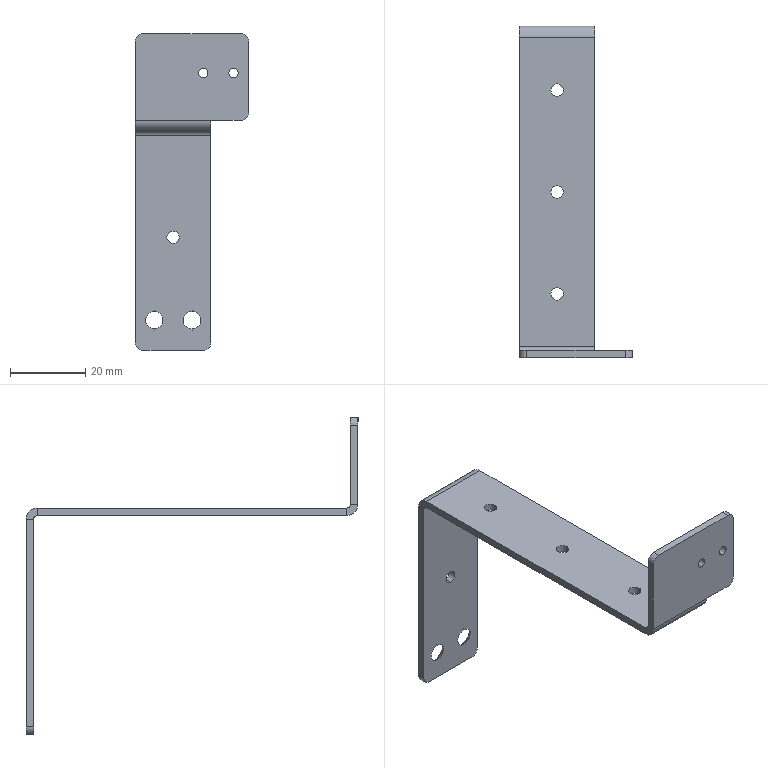Part | STEP file | FBDS-CS-014 | 1 solid | 44 faces | box 30 x 88 x 84 mm | volume 6954 mm3 | cylinder 21 | plane 19 | cone 4 | commonest cylinder face diameters 3.3 x8 4 x5 2.5 x4 2 x2 6 x2
STEP:
#1=CARTESIAN_POINT('',(0.,42.,-28.35));
#2=VERTEX_POINT('',#1);
#3=CARTESIAN_POINT('',(0.,42.,-31.65));
#4=VERTEX_POINT('',#3);
#5=CARTESIAN_POINT('',(0.,42.,-30.));
#6=DIRECTION('',(0.,-1.,0.));
#7=DIRECTION('',(0.,0.,-1.));
#8=AXIS2_PLACEMENT_3D('',#5,#6,#7);
#9=CIRCLE('',#8,1.65);
#10=EDGE_CURVE('',#2,#4,#9,.T.);
#11=ORIENTED_EDGE('',*,*,#10,.T.);
#12=CARTESIAN_POINT('',(0.,44.,-31.65));
#13=VERTEX_POINT('',#12);
#14=CARTESIAN_POINT('',(0.,44.,-31.65));
#15=DIRECTION('',(0.,1.,0.));
#16=VECTOR('',#15,1000.);
#17=LINE('',#14,#16);
#18=EDGE_CURVE('',#4,#13,#17,.T.);
#19=ORIENTED_EDGE('',*,*,#18,.T.);
#20=CARTESIAN_POINT('',(0.,44.,-28.35));
#21=VERTEX_POINT('',#20);
#22=CARTESIAN_POINT('',(0.,44.,-30.));
#23=DIRECTION('',(0.,1.,0.));
#24=DIRECTION('',(0.,0.,1.));
#25=AXIS2_PLACEMENT_3D('',#22,#23,#24);
#26=CIRCLE('',#25,1.65);
#27=EDGE_CURVE('',#13,#21,#26,.T.);
#28=ORIENTED_EDGE('',*,*,#27,.T.);
#29=CARTESIAN_POINT('',(0.,44.,-28.35));
#30=DIRECTION('',(0.,1.,0.));
#31=VECTOR('',#30,1000.);
#32=LINE('',#29,#31);
#33=EDGE_CURVE('',#2,#21,#32,.T.);
#34=ORIENTED_EDGE('',*,*,#33,.F.);
#35=EDGE_LOOP('',(#11,#19,#28,#34));
#36=FACE_OUTER_BOUND('',#35,.T.);
#37=CARTESIAN_POINT('',(0.,44.,-30.));
#38=DIRECTION('',(0.,1.,0.));
#39=DIRECTION('',(0.,0.,1.));
#40=AXIS2_PLACEMENT_3D('',#37,#38,#39);
#41=CYLINDRICAL_SURFACE('',#40,1.65);
#42=ADVANCED_FACE('',(#36),#41,.F.);
#43=CARTESIAN_POINT('',(1.65,27.,-2.));
#44=VERTEX_POINT('',#43);
#45=CARTESIAN_POINT('',(-1.65,27.,-2.));
#46=VERTEX_POINT('',#45);
#47=CARTESIAN_POINT('',(0.,27.,-2.));
#48=DIRECTION('',(0.,0.,-1.));
#49=DIRECTION('',(-1.,0.,0.));
#50=AXIS2_PLACEMENT_3D('',#47,#48,#49);
#51=CIRCLE('',#50,1.65);
#52=EDGE_CURVE('',#44,#46,#51,.T.);
#53=ORIENTED_EDGE('',*,*,#52,.T.);
#54=CARTESIAN_POINT('',(-1.65,27.,0.));
#55=VERTEX_POINT('',#54);
#56=CARTESIAN_POINT('',(-1.65,27.,0.));
#57=DIRECTION('',(0.,0.,1.));
#58=VECTOR('',#57,1000.);
#59=LINE('',#56,#58);
#60=EDGE_CURVE('',#46,#55,#59,.T.);
#61=ORIENTED_EDGE('',*,*,#60,.T.);
#62=CARTESIAN_POINT('',(1.65,27.,0.));
#63=VERTEX_POINT('',#62);
#64=CARTESIAN_POINT('',(0.,27.,0.));
#65=DIRECTION('',(0.,0.,1.));
#66=DIRECTION('',(1.,0.,0.));
#67=AXIS2_PLACEMENT_3D('',#64,#65,#66);
#68=CIRCLE('',#67,1.65);
#69=EDGE_CURVE('',#55,#63,#68,.T.);
#70=ORIENTED_EDGE('',*,*,#69,.T.);
#71=CARTESIAN_POINT('',(1.65,27.,0.));
#72=DIRECTION('',(0.,0.,1.));
#73=VECTOR('',#72,1000.);
#74=LINE('',#71,#73);
#75=EDGE_CURVE('',#44,#63,#74,.T.);
#76=ORIENTED_EDGE('',*,*,#75,.F.);
#77=EDGE_LOOP('',(#53,#61,#70,#76));
#78=FACE_OUTER_BOUND('',#77,.T.);
#79=CARTESIAN_POINT('',(0.,27.,0.));
#80=DIRECTION('',(0.,0.,1.));
#81=DIRECTION('',(1.,0.,0.));
#82=AXIS2_PLACEMENT_3D('',#79,#80,#81);
#83=CYLINDRICAL_SURFACE('',#82,1.65);
#84=ADVANCED_FACE('',(#78),#83,.F.);
#85=CARTESIAN_POINT('',(1.65,0.,-2.));
#86=VERTEX_POINT('',#85);
#87=CARTESIAN_POINT('',(-1.65,0.,-2.));
#88=VERTEX_POINT('',#87);
#89=CARTESIAN_POINT('',(0.,0.,-2.));
#90=DIRECTION('',(0.,0.,-1.));
#91=DIRECTION('',(-1.,0.,0.));
#92=AXIS2_PLACEMENT_3D('',#89,#90,#91);
#93=CIRCLE('',#92,1.65);
#94=EDGE_CURVE('',#86,#88,#93,.T.);
#95=ORIENTED_EDGE('',*,*,#94,.T.);
#96=CARTESIAN_POINT('',(-1.65,0.,0.));
#97=VERTEX_POINT('',#96);
#98=CARTESIAN_POINT('',(-1.65,0.,0.));
#99=DIRECTION('',(0.,0.,1.));
#100=VECTOR('',#99,1000.);
#101=LINE('',#98,#100);
#102=EDGE_CURVE('',#88,#97,#101,.T.);
#103=ORIENTED_EDGE('',*,*,#102,.T.);
#104=CARTESIAN_POINT('',(1.65,0.,0.));
#105=VERTEX_POINT('',#104);
#106=CARTESIAN_POINT('',(0.,0.,0.));
#107=DIRECTION('',(0.,0.,1.));
#108=DIRECTION('',(1.,0.,0.));
#109=AXIS2_PLACEMENT_3D('',#106,#107,#108);
#110=CIRCLE('',#109,1.65);
#111=EDGE_CURVE('',#97,#105,#110,.T.);
#112=ORIENTED_EDGE('',*,*,#111,.T.);
#113=CARTESIAN_POINT('',(1.65,0.,0.));
#114=DIRECTION('',(0.,0.,1.));
#115=VECTOR('',#114,1000.);
#116=LINE('',#113,#115);
#117=EDGE_CURVE('',#86,#105,#116,.T.);
#118=ORIENTED_EDGE('',*,*,#117,.F.);
#119=EDGE_LOOP('',(#95,#103,#112,#118));
#120=FACE_OUTER_BOUND('',#119,.T.);
#121=CARTESIAN_POINT('',(0.,0.,0.));
#122=DIRECTION('',(0.,0.,1.));
#123=DIRECTION('',(1.,0.,0.));
#124=AXIS2_PLACEMENT_3D('',#121,#122,#123);
#125=CYLINDRICAL_SURFACE('',#124,1.65);
#126=ADVANCED_FACE('',(#120),#125,.F.);
#127=CARTESIAN_POINT('',(1.65,-27.,-2.));
#128=VERTEX_POINT('',#127);
#129=CARTESIAN_POINT('',(-1.65,-27.,-2.));
#130=VERTEX_POINT('',#129);
#131=CARTESIAN_POINT('',(0.,-27.,-2.));
#132=DIRECTION('',(0.,0.,-1.));
#133=DIRECTION('',(-1.,0.,0.));
#134=AXIS2_PLACEMENT_3D('',#131,#132,#133);
#135=CIRCLE('',#134,1.65);
#136=EDGE_CURVE('',#128,#130,#135,.T.);
#137=ORIENTED_EDGE('',*,*,#136,.T.);
#138=CARTESIAN_POINT('',(-1.65,-27.,0.));
#139=VERTEX_POINT('',#138);
#140=CARTESIAN_POINT('',(-1.65,-27.,0.));
#141=DIRECTION('',(0.,0.,1.));
#142=VECTOR('',#141,1000.);
#143=LINE('',#140,#142);
#144=EDGE_CURVE('',#130,#139,#143,.T.);
#145=ORIENTED_EDGE('',*,*,#144,.T.);
#146=CARTESIAN_POINT('',(1.65,-27.,0.));
#147=VERTEX_POINT('',#146);
#148=CARTESIAN_POINT('',(0.,-27.,0.));
#149=DIRECTION('',(0.,0.,1.));
#150=DIRECTION('',(1.,0.,0.));
#151=AXIS2_PLACEMENT_3D('',#148,#149,#150);
#152=CIRCLE('',#151,1.65);
#153=EDGE_CURVE('',#139,#147,#152,.T.);
#154=ORIENTED_EDGE('',*,*,#153,.T.);
#155=CARTESIAN_POINT('',(1.65,-27.,0.));
#156=DIRECTION('',(0.,0.,1.));
#157=VECTOR('',#156,1000.);
#158=LINE('',#155,#157);
#159=EDGE_CURVE('',#128,#147,#158,.T.);
#160=ORIENTED_EDGE('',*,*,#159,.F.);
#161=EDGE_LOOP('',(#137,#145,#154,#160));
#162=FACE_OUTER_BOUND('',#161,.T.);
#163=CARTESIAN_POINT('',(0.,-27.,0.));
#164=DIRECTION('',(0.,0.,1.));
#165=DIRECTION('',(1.,0.,0.));
#166=AXIS2_PLACEMENT_3D('',#163,#164,#165);
#167=CYLINDRICAL_SURFACE('',#166,1.65);
#168=ADVANCED_FACE('',(#162),#167,.F.);
#169=CARTESIAN_POINT('',(16.,-44.,12.25));
#170=VERTEX_POINT('',#169);
#171=CARTESIAN_POINT('',(16.,-44.,14.75));
#172=VERTEX_POINT('',#171);
#173=CARTESIAN_POINT('',(16.,-44.,13.5));
#174=DIRECTION('',(0.,1.,0.));
#175=DIRECTION('',(0.,0.,1.));
#176=AXIS2_PLACEMENT_3D('',#173,#174,#175);
#177=CIRCLE('',#176,1.25);
#178=EDGE_CURVE('',#170,#172,#177,.T.);
#179=ORIENTED_EDGE('',*,*,#178,.F.);
#180=CARTESIAN_POINT('',(16.,-42.,12.25));
#181=VERTEX_POINT('',#180);
#182=CARTESIAN_POINT('',(16.,-42.,12.25));
#183=DIRECTION('',(0.,1.,0.));
#184=VECTOR('',#183,1000.);
#185=LINE('',#182,#184);
#186=EDGE_CURVE('',#170,#181,#185,.T.);
#187=ORIENTED_EDGE('',*,*,#186,.T.);
#188=CARTESIAN_POINT('',(16.,-42.,14.75));
#189=VERTEX_POINT('',#188);
#190=CARTESIAN_POINT('',(16.,-42.,13.5));
#191=DIRECTION('',(0.,1.,0.));
#192=DIRECTION('',(0.,0.,1.));
#193=AXIS2_PLACEMENT_3D('',#190,#191,#192);
#194=CIRCLE('',#193,1.25);
#195=EDGE_CURVE('',#181,#189,#194,.T.);
#196=ORIENTED_EDGE('',*,*,#195,.T.);
#197=CARTESIAN_POINT('',(16.,-42.,14.75));
#198=DIRECTION('',(0.,1.,0.));
#199=VECTOR('',#198,1000.);
#200=LINE('',#197,#199);
#201=EDGE_CURVE('',#172,#189,#200,.T.);
#202=ORIENTED_EDGE('',*,*,#201,.F.);
#203=EDGE_LOOP('',(#179,#187,#196,#202));
#204=FACE_OUTER_BOUND('',#203,.T.);
#205=CARTESIAN_POINT('',(16.,-42.,13.5));
#206=DIRECTION('',(0.,1.,0.));
#207=DIRECTION('',(0.,0.,1.));
#208=AXIS2_PLACEMENT_3D('',#205,#206,#207);
#209=CYLINDRICAL_SURFACE('',#208,1.25);
#210=ADVANCED_FACE('',(#204),#209,.F.);
#211=CARTESIAN_POINT('',(8.,-44.,12.25));
#212=VERTEX_POINT('',#211);
#213=CARTESIAN_POINT('',(8.,-44.,14.75));
#214=VERTEX_POINT('',#213);
#215=CARTESIAN_POINT('',(8.,-44.,13.5));
#216=DIRECTION('',(0.,1.,0.));
#217=DIRECTION('',(0.,0.,1.));
#218=AXIS2_PLACEMENT_3D('',#215,#216,#217);
#219=CIRCLE('',#218,1.25);
#220=EDGE_CURVE('',#212,#214,#219,.T.);
#221=ORIENTED_EDGE('',*,*,#220,.F.);
#222=CARTESIAN_POINT('',(8.,-42.,12.25));
#223=VERTEX_POINT('',#222);
#224=CARTESIAN_POINT('',(8.,-42.,12.25));
#225=DIRECTION('',(0.,1.,0.));
#226=VECTOR('',#225,1000.);
#227=LINE('',#224,#226);
#228=EDGE_CURVE('',#212,#223,#227,.T.);
#229=ORIENTED_EDGE('',*,*,#228,.T.);
#230=CARTESIAN_POINT('',(8.,-42.,14.75));
#231=VERTEX_POINT('',#230);
#232=CARTESIAN_POINT('',(8.,-42.,13.5));
#233=DIRECTION('',(0.,1.,0.));
#234=DIRECTION('',(0.,0.,1.));
#235=AXIS2_PLACEMENT_3D('',#232,#233,#234);
#236=CIRCLE('',#235,1.25);
#237=EDGE_CURVE('',#223,#231,#236,.T.);
#238=ORIENTED_EDGE('',*,*,#237,.T.);
#239=CARTESIAN_POINT('',(8.,-42.,14.75));
#240=DIRECTION('',(0.,1.,0.));
#241=VECTOR('',#240,1000.);
#242=LINE('',#239,#241);
#243=EDGE_CURVE('',#214,#231,#242,.T.);
#244=ORIENTED_EDGE('',*,*,#243,.F.);
#245=EDGE_LOOP('',(#221,#229,#238,#244));
#246=FACE_OUTER_BOUND('',#245,.T.);
#247=CARTESIAN_POINT('',(8.,-42.,13.5));
#248=DIRECTION('',(0.,1.,0.));
#249=DIRECTION('',(0.,0.,1.));
#250=AXIS2_PLACEMENT_3D('',#247,#248,#249);
#251=CYLINDRICAL_SURFACE('',#250,1.25);
#252=ADVANCED_FACE('',(#246),#251,.F.);
#253=CARTESIAN_POINT('',(-5.,42.,-49.7));
#254=VERTEX_POINT('',#253);
#255=CARTESIAN_POINT('',(-5.,42.,-54.3));
#256=VERTEX_POINT('',#255);
#257=CARTESIAN_POINT('',(-5.,42.,-52.));
#258=DIRECTION('',(0.,-1.,0.));
#259=DIRECTION('',(0.,0.,-1.));
#260=AXIS2_PLACEMENT_3D('',#257,#258,#259);
#261=CIRCLE('',#260,2.3);
#262=EDGE_CURVE('',#254,#256,#261,.T.);
#263=ORIENTED_EDGE('',*,*,#262,.T.);
#264=CARTESIAN_POINT('',(-5.,44.,-56.3));
#265=VERTEX_POINT('',#264);
#266=CARTESIAN_POINT('',(-5.,44.,-56.3));
#267=DIRECTION('',(0.,0.7071,-0.7071));
#268=VECTOR('',#267,1000.);
#269=LINE('',#266,#268);
#270=EDGE_CURVE('',#256,#265,#269,.T.);
#271=ORIENTED_EDGE('',*,*,#270,.T.);
#272=CARTESIAN_POINT('',(-5.,44.,-47.7));
#273=VERTEX_POINT('',#272);
#274=CARTESIAN_POINT('',(-5.,44.,-52.));
#275=DIRECTION('',(0.,1.,0.));
#276=DIRECTION('',(0.,0.,1.));
#277=AXIS2_PLACEMENT_3D('',#274,#275,#276);
#278=CIRCLE('',#277,4.3);
#279=EDGE_CURVE('',#265,#273,#278,.T.);
#280=ORIENTED_EDGE('',*,*,#279,.T.);
#281=CARTESIAN_POINT('',(-5.,44.,-47.7));
#282=DIRECTION('',(0.,0.7071,0.7071));
#283=VECTOR('',#282,1000.);
#284=LINE('',#281,#283);
#285=EDGE_CURVE('',#254,#273,#284,.T.);
#286=ORIENTED_EDGE('',*,*,#285,.F.);
#287=EDGE_LOOP('',(#263,#271,#280,#286));
#288=FACE_OUTER_BOUND('',#287,.T.);
#289=CARTESIAN_POINT('',(-5.,44.,-52.));
#290=DIRECTION('',(0.,1.,0.));
#291=DIRECTION('',(0.,0.,1.));
#292=AXIS2_PLACEMENT_3D('',#289,#290,#291);
#293=CONICAL_SURFACE('',#292,4.3,0.7854);
#294=ADVANCED_FACE('',(#288),#293,.F.);
#295=CARTESIAN_POINT('',(5.,42.,-49.7));
#296=VERTEX_POINT('',#295);
#297=CARTESIAN_POINT('',(5.,42.,-54.3));
#298=VERTEX_POINT('',#297);
#299=CARTESIAN_POINT('',(5.,42.,-52.));
#300=DIRECTION('',(0.,-1.,0.));
#301=DIRECTION('',(0.,0.,-1.));
#302=AXIS2_PLACEMENT_3D('',#299,#300,#301);
#303=CIRCLE('',#302,2.3);
#304=EDGE_CURVE('',#296,#298,#303,.T.);
#305=ORIENTED_EDGE('',*,*,#304,.T.);
#306=CARTESIAN_POINT('',(5.,44.,-56.3));
#307=VERTEX_POINT('',#306);
#308=CARTESIAN_POINT('',(5.,44.,-56.3));
#309=DIRECTION('',(0.,0.7071,-0.7071));
#310=VECTOR('',#309,1000.);
#311=LINE('',#308,#310);
#312=EDGE_CURVE('',#298,#307,#311,.T.);
#313=ORIENTED_EDGE('',*,*,#312,.T.);
#314=CARTESIAN_POINT('',(5.,44.,-47.7));
#315=VERTEX_POINT('',#314);
#316=CARTESIAN_POINT('',(5.,44.,-52.));
#317=DIRECTION('',(0.,1.,0.));
#318=DIRECTION('',(0.,0.,1.));
#319=AXIS2_PLACEMENT_3D('',#316,#317,#318);
#320=CIRCLE('',#319,4.3);
#321=EDGE_CURVE('',#307,#315,#320,.T.);
#322=ORIENTED_EDGE('',*,*,#321,.T.);
#323=CARTESIAN_POINT('',(5.,44.,-47.7));
#324=DIRECTION('',(0.,0.7071,0.7071));
#325=VECTOR('',#324,1000.);
#326=LINE('',#323,#325);
#327=EDGE_CURVE('',#296,#315,#326,.T.);
#328=ORIENTED_EDGE('',*,*,#327,.F.);
#329=EDGE_LOOP('',(#305,#313,#322,#328));
#330=FACE_OUTER_BOUND('',#329,.T.);
#331=CARTESIAN_POINT('',(5.,44.,-52.));
#332=DIRECTION('',(0.,1.,0.));
#333=DIRECTION('',(0.,0.,1.));
#334=AXIS2_PLACEMENT_3D('',#331,#332,#333);
#335=CONICAL_SURFACE('',#334,4.3,0.7854);
#336=ADVANCED_FACE('',(#330),#335,.F.);
#337=CARTESIAN_POINT('',(10.,-41.,0.));
#338=VERTEX_POINT('',#337);
#339=CARTESIAN_POINT('',(10.,41.,0.));
#340=VERTEX_POINT('',#339);
#341=CARTESIAN_POINT('',(10.,-42.,0.));
#342=DIRECTION('',(0.,1.,0.));
#343=VECTOR('',#342,1000.);
#344=LINE('',#341,#343);
#345=EDGE_CURVE('',#338,#340,#344,.T.);
#346=ORIENTED_EDGE('',*,*,#345,.F.);
#347=CARTESIAN_POINT('',(10.,-41.,-2.));
#348=VERTEX_POINT('',#347);
#349=CARTESIAN_POINT('',(10.,-41.,0.));
#350=DIRECTION('',(0.,0.,-1.));
#351=VECTOR('',#350,1000.);
#352=LINE('',#349,#351);
#353=EDGE_CURVE('',#338,#348,#352,.T.);
#354=ORIENTED_EDGE('',*,*,#353,.T.);
#355=CARTESIAN_POINT('',(10.,41.,-2.));
#356=VERTEX_POINT('',#355);
#357=CARTESIAN_POINT('',(10.,-42.,-2.));
#358=DIRECTION('',(0.,1.,0.));
#359=VECTOR('',#358,1000.);
#360=LINE('',#357,#359);
#361=EDGE_CURVE('',#348,#356,#360,.T.);
#362=ORIENTED_EDGE('',*,*,#361,.T.);
#363=CARTESIAN_POINT('',(10.,41.,-2.));
#364=DIRECTION('',(0.,0.,1.));
#365=VECTOR('',#364,1000.);
#366=LINE('',#363,#365);
#367=EDGE_CURVE('',#356,#340,#366,.T.);
#368=ORIENTED_EDGE('',*,*,#367,.T.);
#369=EDGE_LOOP('',(#346,#354,#362,#368));
#370=FACE_OUTER_BOUND('',#369,.T.);
#371=CARTESIAN_POINT('',(10.,-42.,-2.));
#372=DIRECTION('',(1.,0.,0.));
#373=DIRECTION('',(0.,0.,-1.));
#374=AXIS2_PLACEMENT_3D('',#371,#372,#373);
#375=PLANE('',#374);
#376=ADVANCED_FACE('',(#370),#375,.T.);
#377=ORIENTED_EDGE('',*,*,#52,.F.);
#378=CARTESIAN_POINT('',(0.,27.,-2.));
#379=DIRECTION('',(0.,0.,-1.));
#380=DIRECTION('',(-1.,0.,0.));
#381=AXIS2_PLACEMENT_3D('',#378,#379,#380);
#382=CIRCLE('',#381,1.65);
#383=EDGE_CURVE('',#46,#44,#382,.T.);
#384=ORIENTED_EDGE('',*,*,#383,.F.);
#385=EDGE_LOOP('',(#377,#384));
#386=FACE_BOUND('',#385,.T.);
#387=ORIENTED_EDGE('',*,*,#94,.F.);
#388=CARTESIAN_POINT('',(0.,0.,-2.));
#389=DIRECTION('',(0.,0.,-1.));
#390=DIRECTION('',(-1.,0.,0.));
#391=AXIS2_PLACEMENT_3D('',#388,#389,#390);
#392=CIRCLE('',#391,1.65);
#393=EDGE_CURVE('',#88,#86,#392,.T.);
#394=ORIENTED_EDGE('',*,*,#393,.F.);
#395=EDGE_LOOP('',(#387,#394));
#396=FACE_BOUND('',#395,.T.);
#397=ORIENTED_EDGE('',*,*,#136,.F.);
#398=CARTESIAN_POINT('',(0.,-27.,-2.));
#399=DIRECTION('',(0.,0.,-1.));
#400=DIRECTION('',(-1.,0.,0.));
#401=AXIS2_PLACEMENT_3D('',#398,#399,#400);
#402=CIRCLE('',#401,1.65);
#403=EDGE_CURVE('',#130,#128,#402,.T.);
#404=ORIENTED_EDGE('',*,*,#403,.F.);
#405=EDGE_LOOP('',(#397,#404));
#406=FACE_BOUND('',#405,.T.);
#407=ORIENTED_EDGE('',*,*,#361,.F.);
#408=CARTESIAN_POINT('',(-10.,-41.,-2.));
#409=VERTEX_POINT('',#408);
#410=CARTESIAN_POINT('',(10.,-41.,-2.));
#411=DIRECTION('',(-1.,0.,0.));
#412=VECTOR('',#411,1000.);
#413=LINE('',#410,#412);
#414=EDGE_CURVE('',#348,#409,#413,.T.);
#415=ORIENTED_EDGE('',*,*,#414,.T.);
#416=CARTESIAN_POINT('',(-10.,41.,-2.));
#417=VERTEX_POINT('',#416);
#418=CARTESIAN_POINT('',(-10.,-42.,-2.));
#419=DIRECTION('',(0.,-1.,0.));
#420=VECTOR('',#419,1000.);
#421=LINE('',#418,#420);
#422=EDGE_CURVE('',#417,#409,#421,.T.);
#423=ORIENTED_EDGE('',*,*,#422,.F.);
#424=CARTESIAN_POINT('',(10.,41.,-2.));
#425=DIRECTION('',(-1.,0.,0.));
#426=VECTOR('',#425,1000.);
#427=LINE('',#424,#426);
#428=EDGE_CURVE('',#356,#417,#427,.T.);
#429=ORIENTED_EDGE('',*,*,#428,.F.);
#430=EDGE_LOOP('',(#407,#415,#423,#429));
#431=FACE_OUTER_BOUND('',#430,.T.);
#432=CARTESIAN_POINT('',(0.,0.,-2.));
#433=DIRECTION('',(0.,0.,-1.));
#434=DIRECTION('',(-1.,0.,0.));
#435=AXIS2_PLACEMENT_3D('',#432,#433,#434);
#436=PLANE('',#435);
#437=ADVANCED_FACE('',(#386,#396,#406,#431),#436,.T.);
#438=CARTESIAN_POINT('',(0.,27.,0.));
#439=DIRECTION('',(0.,0.,1.));
#440=DIRECTION('',(1.,0.,0.));
#441=AXIS2_PLACEMENT_3D('',#438,#439,#440);
#442=CIRCLE('',#441,1.65);
#443=EDGE_CURVE('',#63,#55,#442,.T.);
#444=ORIENTED_EDGE('',*,*,#443,.F.);
#445=ORIENTED_EDGE('',*,*,#69,.F.);
#446=EDGE_LOOP('',(#444,#445));
#447=FACE_BOUND('',#446,.T.);
#448=CARTESIAN_POINT('',(0.,0.,0.));
#449=DIRECTION('',(0.,0.,1.));
#450=DIRECTION('',(1.,0.,0.));
#451=AXIS2_PLACEMENT_3D('',#448,#449,#450);
#452=CIRCLE('',#451,1.65);
#453=EDGE_CURVE('',#105,#97,#452,.T.);
#454=ORIENTED_EDGE('',*,*,#453,.F.);
#455=ORIENTED_EDGE('',*,*,#111,.F.);
#456=EDGE_LOOP('',(#454,#455));
#457=FACE_BOUND('',#456,.T.);
#458=CARTESIAN_POINT('',(0.,-27.,0.));
#459=DIRECTION('',(0.,0.,1.));
#460=DIRECTION('',(1.,0.,0.));
#461=AXIS2_PLACEMENT_3D('',#458,#459,#460);
#462=CIRCLE('',#461,1.65);
#463=EDGE_CURVE('',#147,#139,#462,.T.);
#464=ORIENTED_EDGE('',*,*,#463,.F.);
#465=ORIENTED_EDGE('',*,*,#153,.F.);
#466=EDGE_LOOP('',(#464,#465));
#467=FACE_BOUND('',#466,.T.);
#468=CARTESIAN_POINT('',(-10.,-41.,0.));
#469=VERTEX_POINT('',#468);
#470=CARTESIAN_POINT('',(10.,-41.,0.));
#471=DIRECTION('',(-1.,0.,0.));
#472=VECTOR('',#471,1000.);
#473=LINE('',#470,#472);
#474=EDGE_CURVE('',#338,#469,#473,.T.);
#475=ORIENTED_EDGE('',*,*,#474,.F.);
#476=ORIENTED_EDGE('',*,*,#345,.T.);
#477=CARTESIAN_POINT('',(-10.,41.,0.));
#478=VERTEX_POINT('',#477);
#479=CARTESIAN_POINT('',(10.,41.,0.));
#480=DIRECTION('',(-1.,0.,0.));
#481=VECTOR('',#480,1000.);
#482=LINE('',#479,#481);
#483=EDGE_CURVE('',#340,#478,#482,.T.);
#484=ORIENTED_EDGE('',*,*,#483,.T.);
#485=CARTESIAN_POINT('',(-10.,-42.,0.));
#486=DIRECTION('',(0.,-1.,0.));
#487=VECTOR('',#486,1000.);
#488=LINE('',#485,#487);
#489=EDGE_CURVE('',#478,#469,#488,.T.);
#490=ORIENTED_EDGE('',*,*,#489,.T.);
#491=EDGE_LOOP('',(#475,#476,#484,#490));
#492=FACE_OUTER_BOUND('',#491,.T.);
#493=CARTESIAN_POINT('',(0.,0.,0.));
#494=DIRECTION('',(0.,0.,-1.));
#495=DIRECTION('',(-1.,0.,0.));
#496=AXIS2_PLACEMENT_3D('',#493,#494,#495);
#497=PLANE('',#496);
#498=ADVANCED_FACE('',(#447,#457,#467,#492),#497,.F.);
#499=CARTESIAN_POINT('',(-10.,-41.,0.));
#500=DIRECTION('',(0.,0.,-1.));
#501=VECTOR('',#500,1000.);
#502=LINE('',#499,#501);
#503=EDGE_CURVE('',#469,#409,#502,.T.);
#504=ORIENTED_EDGE('',*,*,#503,.F.);
#505=ORIENTED_EDGE('',*,*,#489,.F.);
#506=CARTESIAN_POINT('',(-10.,41.,-2.));
#507=DIRECTION('',(0.,0.,1.));
#508=VECTOR('',#507,1000.);
#509=LINE('',#506,#508);
#510=EDGE_CURVE('',#417,#478,#509,.T.);
#511=ORIENTED_EDGE('',*,*,#510,.F.);
#512=ORIENTED_EDGE('',*,*,#422,.T.);
#513=EDGE_LOOP('',(#504,#505,#511,#512));
#514=FACE_OUTER_BOUND('',#513,.T.);
#515=CARTESIAN_POINT('',(-10.,-42.,-2.));
#516=DIRECTION('',(-1.,0.,0.));
#517=DIRECTION('',(0.,0.,1.));
#518=AXIS2_PLACEMENT_3D('',#515,#516,#517);
#519=PLANE('',#518);
#520=ADVANCED_FACE('',(#514),#519,.T.);
#521=CARTESIAN_POINT('',(-10.,42.,-3.));
#522=VERTEX_POINT('',#521);
#523=CARTESIAN_POINT('',(-10.,44.,-3.));
#524=VERTEX_POINT('',#523);
#525=CARTESIAN_POINT('',(-10.,42.,-3.));
#526=DIRECTION('',(0.,1.,0.));
#527=VECTOR('',#526,1000.);
#528=LINE('',#525,#527);
#529=EDGE_CURVE('',#522,#524,#528,.T.);
#530=ORIENTED_EDGE('',*,*,#529,.F.);
#531=CARTESIAN_POINT('',(-10.,41.,-3.));
#532=DIRECTION('',(-1.,0.,0.));
#533=DIRECTION('',(0.,0.,-1.));
#534=AXIS2_PLACEMENT_3D('',#531,#532,#533);
#535=CIRCLE('',#534,1.);
#536=EDGE_CURVE('',#417,#522,#535,.T.);
#537=ORIENTED_EDGE('',*,*,#536,.F.);
#538=ORIENTED_EDGE('',*,*,#510,.T.);
#539=CARTESIAN_POINT('',(-10.,41.,-3.));
#540=DIRECTION('',(-1.,0.,0.));
#541=DIRECTION('',(0.,0.,-1.));
#542=AXIS2_PLACEMENT_3D('',#539,#540,#541);
#543=CIRCLE('',#542,3.);
#544=EDGE_CURVE('',#478,#524,#543,.T.);
#545=ORIENTED_EDGE('',*,*,#544,.T.);
#546=EDGE_LOOP('',(#530,#537,#538,#545));
#547=FACE_OUTER_BOUND('',#546,.T.);
#548=CARTESIAN_POINT('',(-10.,41.,-3.));
#549=DIRECTION('',(-1.,0.,0.));
#550=DIRECTION('',(0.,0.,1.));
#551=AXIS2_PLACEMENT_3D('',#548,#549,#550);
#552=PLANE('',#551);
#553=ADVANCED_FACE('',(#547),#552,.T.);
#554=CARTESIAN_POINT('',(10.,42.,-3.));
#555=VERTEX_POINT('',#554);
#556=CARTESIAN_POINT('',(10.,41.,-3.));
#557=DIRECTION('',(1.,0.,0.));
#558=DIRECTION('',(0.,0.,-1.));
#559=AXIS2_PLACEMENT_3D('',#556,#557,#558);
#560=CIRCLE('',#559,1.);
#561=EDGE_CURVE('',#555,#356,#560,.T.);
#562=ORIENTED_EDGE('',*,*,#561,.F.);
#563=CARTESIAN_POINT('',(10.,44.,-3.));
#564=VERTEX_POINT('',#563);
#565=CARTESIAN_POINT('',(10.,42.,-3.));
#566=DIRECTION('',(0.,1.,0.));
#567=VECTOR('',#566,1000.);
#568=LINE('',#565,#567);
#569=EDGE_CURVE('',#555,#564,#568,.T.);
#570=ORIENTED_EDGE('',*,*,#569,.T.);
#571=CARTESIAN_POINT('',(10.,41.,-3.));
#572=DIRECTION('',(1.,0.,0.));
#573=DIRECTION('',(0.,0.,-1.));
#574=AXIS2_PLACEMENT_3D('',#571,#572,#573);
#575=CIRCLE('',#574,3.);
#576=EDGE_CURVE('',#564,#340,#575,.T.);
#577=ORIENTED_EDGE('',*,*,#576,.T.);
#578=ORIENTED_EDGE('',*,*,#367,.F.);
#579=EDGE_LOOP('',(#562,#570,#577,#578));
#580=FACE_OUTER_BOUND('',#579,.T.);
#581=CARTESIAN_POINT('',(10.,41.,-3.));
#582=DIRECTION('',(-1.,0.,0.));
#583=DIRECTION('',(0.,0.,1.));
#584=AXIS2_PLACEMENT_3D('',#581,#582,#583);
#585=PLANE('',#584);
#586=ADVANCED_FACE('',(#580),#585,.F.);
#587=ORIENTED_EDGE('',*,*,#483,.F.);
#588=ORIENTED_EDGE('',*,*,#576,.F.);
#589=CARTESIAN_POINT('',(0.,44.,-3.));
#590=DIRECTION('',(-1.,0.,0.));
#591=VECTOR('',#590,1000.);
#592=LINE('',#589,#591);
#593=EDGE_CURVE('',#564,#524,#592,.T.);
#594=ORIENTED_EDGE('',*,*,#593,.T.);
#595=ORIENTED_EDGE('',*,*,#544,.F.);
#596=EDGE_LOOP('',(#587,#588,#594,#595));
#597=FACE_OUTER_BOUND('',#596,.T.);
#598=CARTESIAN_POINT('',(10.,41.,-3.));
#599=DIRECTION('',(1.,0.,0.));
#600=DIRECTION('',(0.,1.,0.));
#601=AXIS2_PLACEMENT_3D('',#598,#599,#600);
#602=CYLINDRICAL_SURFACE('',#601,3.);
#603=ADVANCED_FACE('',(#597),#602,.T.);
#604=ORIENTED_EDGE('',*,*,#428,.T.);
#605=ORIENTED_EDGE('',*,*,#536,.T.);
#606=CARTESIAN_POINT('',(-10.,42.,-3.));
#607=DIRECTION('',(1.,0.,0.));
#608=VECTOR('',#607,1000.);
#609=LINE('',#606,#608);
#610=EDGE_CURVE('',#522,#555,#609,.T.);
#611=ORIENTED_EDGE('',*,*,#610,.T.);
#612=ORIENTED_EDGE('',*,*,#561,.T.);
#613=EDGE_LOOP('',(#604,#605,#611,#612));
#614=FACE_OUTER_BOUND('',#613,.T.);
#615=CARTESIAN_POINT('',(10.,41.,-3.));
#616=DIRECTION('',(1.,0.,0.));
#617=DIRECTION('',(0.,1.,0.));
#618=AXIS2_PLACEMENT_3D('',#615,#616,#617);
#619=CYLINDRICAL_SURFACE('',#618,1.);
#620=ADVANCED_FACE('',(#614),#619,.F.);
#621=CARTESIAN_POINT('',(10.,42.,-58.));
#622=VERTEX_POINT('',#621);
#623=CARTESIAN_POINT('',(10.,42.,-60.));
#624=DIRECTION('',(0.,0.,-1.));
#625=VECTOR('',#624,1000.);
#626=LINE('',#623,#625);
#627=EDGE_CURVE('',#555,#622,#626,.T.);
#628=ORIENTED_EDGE('',*,*,#627,.T.);
#629=CARTESIAN_POINT('',(10.,44.,-58.));
#630=VERTEX_POINT('',#629);
#631=CARTESIAN_POINT('',(10.,44.,-58.));
#632=DIRECTION('',(0.,1.,0.));
#633=VECTOR('',#632,1000.);
#634=LINE('',#631,#633);
#635=EDGE_CURVE('',#622,#630,#634,.T.);
#636=ORIENTED_EDGE('',*,*,#635,.T.);
#637=CARTESIAN_POINT('',(10.,44.,-60.));
#638=DIRECTION('',(0.,0.,-1.));
#639=VECTOR('',#638,1000.);
#640=LINE('',#637,#639);
#641=EDGE_CURVE('',#564,#630,#640,.T.);
#642=ORIENTED_EDGE('',*,*,#641,.F.);
#643=ORIENTED_EDGE('',*,*,#569,.F.);
#644=EDGE_LOOP('',(#628,#636,#642,#643));
#645=FACE_OUTER_BOUND('',#644,.T.);
#646=CARTESIAN_POINT('',(10.,44.,-60.));
#647=DIRECTION('',(-1.,0.,0.));
#648=DIRECTION('',(0.,0.,1.));
#649=AXIS2_PLACEMENT_3D('',#646,#647,#648);
#650=PLANE('',#649);
#651=ADVANCED_FACE('',(#645),#650,.F.);
#652=CARTESIAN_POINT('',(-10.,44.,-58.));
#653=VERTEX_POINT('',#652);
#654=CARTESIAN_POINT('',(-10.,44.,-2.));
#655=DIRECTION('',(0.,0.,1.));
#656=VECTOR('',#655,1000.);
#657=LINE('',#654,#656);
#658=EDGE_CURVE('',#653,#524,#657,.T.);
#659=ORIENTED_EDGE('',*,*,#658,.F.);
#660=CARTESIAN_POINT('',(-10.,42.,-58.));
#661=VERTEX_POINT('',#660);
#662=CARTESIAN_POINT('',(-10.,44.,-58.));
#663=DIRECTION('',(0.,-1.,0.));
#664=VECTOR('',#663,1000.);
#665=LINE('',#662,#664);
#666=EDGE_CURVE('',#653,#661,#665,.T.);
#667=ORIENTED_EDGE('',*,*,#666,.T.);
#668=CARTESIAN_POINT('',(-10.,42.,-2.));
#669=DIRECTION('',(0.,0.,1.));
#670=VECTOR('',#669,1000.);
#671=LINE('',#668,#670);
#672=EDGE_CURVE('',#661,#522,#671,.T.);
#673=ORIENTED_EDGE('',*,*,#672,.T.);
#674=ORIENTED_EDGE('',*,*,#529,.T.);
#675=EDGE_LOOP('',(#659,#667,#673,#674));
#676=FACE_OUTER_BOUND('',#675,.T.);
#677=CARTESIAN_POINT('',(-10.,44.,-2.));
#678=DIRECTION('',(1.,0.,0.));
#679=DIRECTION('',(0.,0.,-1.));
#680=AXIS2_PLACEMENT_3D('',#677,#678,#679);
#681=PLANE('',#680);
#682=ADVANCED_FACE('',(#676),#681,.F.);
#683=CARTESIAN_POINT('',(0.,44.,-30.));
#684=DIRECTION('',(0.,1.,0.));
#685=DIRECTION('',(0.,0.,1.));
#686=AXIS2_PLACEMENT_3D('',#683,#684,#685);
#687=CIRCLE('',#686,1.65);
#688=EDGE_CURVE('',#21,#13,#687,.T.);
#689=ORIENTED_EDGE('',*,*,#688,.F.);
#690=ORIENTED_EDGE('',*,*,#27,.F.);
#691=EDGE_LOOP('',(#689,#690));
#692=FACE_BOUND('',#691,.T.);
#693=CARTESIAN_POINT('',(-5.,44.,-52.));
#694=DIRECTION('',(0.,1.,0.));
#695=DIRECTION('',(0.,0.,1.));
#696=AXIS2_PLACEMENT_3D('',#693,#694,#695);
#697=CIRCLE('',#696,4.3);
#698=EDGE_CURVE('',#273,#265,#697,.T.);
#699=ORIENTED_EDGE('',*,*,#698,.F.);
#700=ORIENTED_EDGE('',*,*,#279,.F.);
#701=EDGE_LOOP('',(#699,#700));
#702=FACE_BOUND('',#701,.T.);
#703=CARTESIAN_POINT('',(5.,44.,-52.));
#704=DIRECTION('',(0.,1.,0.));
#705=DIRECTION('',(0.,0.,1.));
#706=AXIS2_PLACEMENT_3D('',#703,#704,#705);
#707=CIRCLE('',#706,4.3);
#708=EDGE_CURVE('',#315,#307,#707,.T.);
#709=ORIENTED_EDGE('',*,*,#708,.F.);
#710=ORIENTED_EDGE('',*,*,#321,.F.);
#711=EDGE_LOOP('',(#709,#710));
#712=FACE_BOUND('',#711,.T.);
#713=ORIENTED_EDGE('',*,*,#641,.T.);
#714=CARTESIAN_POINT('',(8.,44.,-60.));
#715=VERTEX_POINT('',#714);
#716=CARTESIAN_POINT('',(8.,44.,-58.));
#717=DIRECTION('',(0.,1.,0.));
#718=DIRECTION('',(0.,0.,-1.));
#719=AXIS2_PLACEMENT_3D('',#716,#717,#718);
#720=CIRCLE('',#719,2.);
#721=EDGE_CURVE('',#630,#715,#720,.T.);
#722=ORIENTED_EDGE('',*,*,#721,.T.);
#723=CARTESIAN_POINT('',(-8.,44.,-60.));
#724=VERTEX_POINT('',#723);
#725=CARTESIAN_POINT('',(-10.,44.,-60.));
#726=DIRECTION('',(-1.,0.,0.));
#727=VECTOR('',#726,1000.);
#728=LINE('',#725,#727);
#729=EDGE_CURVE('',#715,#724,#728,.T.);
#730=ORIENTED_EDGE('',*,*,#729,.T.);
#731=CARTESIAN_POINT('',(-8.,44.,-58.));
#732=DIRECTION('',(0.,1.,0.));
#733=DIRECTION('',(0.,0.,-1.));
#734=AXIS2_PLACEMENT_3D('',#731,#732,#733);
#735=CIRCLE('',#734,2.);
#736=EDGE_CURVE('',#724,#653,#735,.T.);
#737=ORIENTED_EDGE('',*,*,#736,.T.);
#738=ORIENTED_EDGE('',*,*,#658,.T.);
#739=ORIENTED_EDGE('',*,*,#593,.F.);
#740=EDGE_LOOP('',(#713,#722,#730,#737,#738,#739));
#741=FACE_OUTER_BOUND('',#740,.T.);
#742=CARTESIAN_POINT('',(0.,44.,0.));
#743=DIRECTION('',(0.,-1.,0.));
#744=DIRECTION('',(0.,0.,-1.));
#745=AXIS2_PLACEMENT_3D('',#742,#743,#744);
#746=PLANE('',#745);
#747=ADVANCED_FACE('',(#692,#702,#712,#741),#746,.F.);
#748=ORIENTED_EDGE('',*,*,#10,.F.);
#749=CARTESIAN_POINT('',(0.,42.,-30.));
#750=DIRECTION('',(0.,-1.,0.));
#751=DIRECTION('',(0.,0.,-1.));
#752=AXIS2_PLACEMENT_3D('',#749,#750,#751);
#753=CIRCLE('',#752,1.65);
#754=EDGE_CURVE('',#4,#2,#753,.T.);
#755=ORIENTED_EDGE('',*,*,#754,.F.);
#756=EDGE_LOOP('',(#748,#755));
#757=FACE_BOUND('',#756,.T.);
#758=ORIENTED_EDGE('',*,*,#262,.F.);
#759=CARTESIAN_POINT('',(-5.,42.,-52.));
#760=DIRECTION('',(0.,-1.,0.));
#761=DIRECTION('',(0.,0.,-1.));
#762=AXIS2_PLACEMENT_3D('',#759,#760,#761);
#763=CIRCLE('',#762,2.3);
#764=EDGE_CURVE('',#256,#254,#763,.T.);
#765=ORIENTED_EDGE('',*,*,#764,.F.);
#766=EDGE_LOOP('',(#758,#765));
#767=FACE_BOUND('',#766,.T.);
#768=ORIENTED_EDGE('',*,*,#304,.F.);
#769=CARTESIAN_POINT('',(5.,42.,-52.));
#770=DIRECTION('',(0.,-1.,0.));
#771=DIRECTION('',(0.,0.,-1.));
#772=AXIS2_PLACEMENT_3D('',#769,#770,#771);
#773=CIRCLE('',#772,2.3);
#774=EDGE_CURVE('',#298,#296,#773,.T.);
#775=ORIENTED_EDGE('',*,*,#774,.F.);
#776=EDGE_LOOP('',(#768,#775));
#777=FACE_BOUND('',#776,.T.);
#778=CARTESIAN_POINT('',(8.,42.,-60.));
#779=VERTEX_POINT('',#778);
#780=CARTESIAN_POINT('',(-8.,42.,-60.));
#781=VERTEX_POINT('',#780);
#782=CARTESIAN_POINT('',(-10.,42.,-60.));
#783=DIRECTION('',(-1.,0.,0.));
#784=VECTOR('',#783,1000.);
#785=LINE('',#782,#784);
#786=EDGE_CURVE('',#779,#781,#785,.T.);
#787=ORIENTED_EDGE('',*,*,#786,.F.);
#788=CARTESIAN_POINT('',(8.,42.,-58.));
#789=DIRECTION('',(0.,-1.,0.));
#790=DIRECTION('',(0.,0.,-1.));
#791=AXIS2_PLACEMENT_3D('',#788,#789,#790);
#792=CIRCLE('',#791,2.);
#793=EDGE_CURVE('',#779,#622,#792,.T.);
#794=ORIENTED_EDGE('',*,*,#793,.T.);
#795=ORIENTED_EDGE('',*,*,#627,.F.);
#796=ORIENTED_EDGE('',*,*,#610,.F.);
#797=ORIENTED_EDGE('',*,*,#672,.F.);
#798=CARTESIAN_POINT('',(-8.,42.,-58.));
#799=DIRECTION('',(0.,-1.,0.));
#800=DIRECTION('',(0.,0.,-1.));
#801=AXIS2_PLACEMENT_3D('',#798,#799,#800);
#802=CIRCLE('',#801,2.);
#803=EDGE_CURVE('',#661,#781,#802,.T.);
#804=ORIENTED_EDGE('',*,*,#803,.T.);
#805=EDGE_LOOP('',(#787,#794,#795,#796,#797,#804));
#806=FACE_OUTER_BOUND('',#805,.T.);
#807=CARTESIAN_POINT('',(0.,42.,0.));
#808=DIRECTION('',(0.,-1.,0.));
#809=DIRECTION('',(0.,0.,-1.));
#810=AXIS2_PLACEMENT_3D('',#807,#808,#809);
#811=PLANE('',#810);
#812=ADVANCED_FACE('',(#757,#767,#777,#806),#811,.T.);
#813=ORIENTED_EDGE('',*,*,#729,.F.);
#814=CARTESIAN_POINT('',(8.,44.,-60.));
#815=DIRECTION('',(0.,-1.,0.));
#816=VECTOR('',#815,1000.);
#817=LINE('',#814,#816);
#818=EDGE_CURVE('',#715,#779,#817,.T.);
#819=ORIENTED_EDGE('',*,*,#818,.T.);
#820=ORIENTED_EDGE('',*,*,#786,.T.);
#821=CARTESIAN_POINT('',(-8.,44.,-60.));
#822=DIRECTION('',(0.,1.,0.));
#823=VECTOR('',#822,1000.);
#824=LINE('',#821,#823);
#825=EDGE_CURVE('',#781,#724,#824,.T.);
#826=ORIENTED_EDGE('',*,*,#825,.T.);
#827=EDGE_LOOP('',(#813,#819,#820,#826));
#828=FACE_OUTER_BOUND('',#827,.T.);
#829=CARTESIAN_POINT('',(-10.,44.,-60.));
#830=DIRECTION('',(0.,0.,1.));
#831=DIRECTION('',(0.,-1.,0.));
#832=AXIS2_PLACEMENT_3D('',#829,#830,#831);
#833=PLANE('',#832);
#834=ADVANCED_FACE('',(#828),#833,.F.);
#835=CARTESIAN_POINT('',(-10.,-42.,1.));
#836=VERTEX_POINT('',#835);
#837=CARTESIAN_POINT('',(-10.,-44.,1.));
#838=VERTEX_POINT('',#837);
#839=CARTESIAN_POINT('',(-10.,-42.,1.));
#840=DIRECTION('',(0.,-1.,0.));
#841=VECTOR('',#840,1000.);
#842=LINE('',#839,#841);
#843=EDGE_CURVE('',#836,#838,#842,.T.);
#844=ORIENTED_EDGE('',*,*,#843,.F.);
#845=CARTESIAN_POINT('',(-10.,-41.,1.));
#846=DIRECTION('',(-1.,0.,0.));
#847=DIRECTION('',(0.,0.,-1.));
#848=AXIS2_PLACEMENT_3D('',#845,#846,#847);
#849=CIRCLE('',#848,1.);
#850=EDGE_CURVE('',#469,#836,#849,.T.);
#851=ORIENTED_EDGE('',*,*,#850,.F.);
#852=ORIENTED_EDGE('',*,*,#503,.T.);
#853=CARTESIAN_POINT('',(-10.,-41.,1.));
#854=DIRECTION('',(-1.,0.,0.));
#855=DIRECTION('',(0.,0.,-1.));
#856=AXIS2_PLACEMENT_3D('',#853,#854,#855);
#857=CIRCLE('',#856,3.);
#858=EDGE_CURVE('',#409,#838,#857,.T.);
#859=ORIENTED_EDGE('',*,*,#858,.T.);
#860=EDGE_LOOP('',(#844,#851,#852,#859));
#861=FACE_OUTER_BOUND('',#860,.T.);
#862=CARTESIAN_POINT('',(-10.,-41.,1.));
#863=DIRECTION('',(-1.,0.,0.));
#864=DIRECTION('',(0.,0.,1.));
#865=AXIS2_PLACEMENT_3D('',#862,#863,#864);
#866=PLANE('',#865);
#867=ADVANCED_FACE('',(#861),#866,.T.);
#868=CARTESIAN_POINT('',(10.,-42.,1.));
#869=VERTEX_POINT('',#868);
#870=CARTESIAN_POINT('',(10.,-41.,1.));
#871=DIRECTION('',(1.,0.,0.));
#872=DIRECTION('',(0.,0.,-1.));
#873=AXIS2_PLACEMENT_3D('',#870,#871,#872);
#874=CIRCLE('',#873,1.);
#875=EDGE_CURVE('',#869,#338,#874,.T.);
#876=ORIENTED_EDGE('',*,*,#875,.F.);
#877=CARTESIAN_POINT('',(10.,-44.,1.));
#878=VERTEX_POINT('',#877);
#879=CARTESIAN_POINT('',(10.,-42.,1.));
#880=DIRECTION('',(0.,-1.,0.));
#881=VECTOR('',#880,1000.);
#882=LINE('',#879,#881);
#883=EDGE_CURVE('',#869,#878,#882,.T.);
#884=ORIENTED_EDGE('',*,*,#883,.T.);
#885=CARTESIAN_POINT('',(10.,-41.,1.));
#886=DIRECTION('',(1.,0.,0.));
#887=DIRECTION('',(0.,0.,-1.));
#888=AXIS2_PLACEMENT_3D('',#885,#886,#887);
#889=CIRCLE('',#888,3.);
#890=EDGE_CURVE('',#878,#348,#889,.T.);
#891=ORIENTED_EDGE('',*,*,#890,.T.);
#892=ORIENTED_EDGE('',*,*,#353,.F.);
#893=EDGE_LOOP('',(#876,#884,#891,#892));
#894=FACE_OUTER_BOUND('',#893,.T.);
#895=CARTESIAN_POINT('',(10.,-41.,1.));
#896=DIRECTION('',(-1.,0.,0.));
#897=DIRECTION('',(0.,0.,1.));
#898=AXIS2_PLACEMENT_3D('',#895,#896,#897);
#899=PLANE('',#898);
#900=ADVANCED_FACE('',(#894),#899,.F.);
#901=ORIENTED_EDGE('',*,*,#414,.F.);
#902=ORIENTED_EDGE('',*,*,#890,.F.);
#903=CARTESIAN_POINT('',(10.,-44.,1.));
#904=DIRECTION('',(1.,0.,0.));
#905=VECTOR('',#904,1000.);
#906=LINE('',#903,#905);
#907=EDGE_CURVE('',#838,#878,#906,.T.);
#908=ORIENTED_EDGE('',*,*,#907,.F.);
#909=ORIENTED_EDGE('',*,*,#858,.F.);
#910=EDGE_LOOP('',(#901,#902,#908,#909));
#911=FACE_OUTER_BOUND('',#910,.T.);
#912=CARTESIAN_POINT('',(10.,-41.,1.));
#913=DIRECTION('',(1.,0.,0.));
#914=DIRECTION('',(0.,-1.,0.));
#915=AXIS2_PLACEMENT_3D('',#912,#913,#914);
#916=CYLINDRICAL_SURFACE('',#915,3.);
#917=ADVANCED_FACE('',(#911),#916,.T.);
#918=ORIENTED_EDGE('',*,*,#474,.T.);
#919=ORIENTED_EDGE('',*,*,#850,.T.);
#920=CARTESIAN_POINT('',(-10.,-42.,1.));
#921=DIRECTION('',(1.,0.,0.));
#922=VECTOR('',#921,1000.);
#923=LINE('',#920,#922);
#924=EDGE_CURVE('',#836,#869,#923,.T.);
#925=ORIENTED_EDGE('',*,*,#924,.T.);
#926=ORIENTED_EDGE('',*,*,#875,.T.);
#927=EDGE_LOOP('',(#918,#919,#925,#926));
#928=FACE_OUTER_BOUND('',#927,.T.);
#929=CARTESIAN_POINT('',(10.,-41.,1.));
#930=DIRECTION('',(1.,0.,0.));
#931=DIRECTION('',(0.,-1.,0.));
#932=AXIS2_PLACEMENT_3D('',#929,#930,#931);
#933=CYLINDRICAL_SURFACE('',#932,1.);
#934=ADVANCED_FACE('',(#928),#933,.F.);
#935=CARTESIAN_POINT('',(18.,-42.,1.));
#936=VERTEX_POINT('',#935);
#937=CARTESIAN_POINT('',(-10.,-42.,1.));
#938=DIRECTION('',(1.,0.,0.));
#939=VECTOR('',#938,1000.);
#940=LINE('',#937,#939);
#941=EDGE_CURVE('',#869,#936,#940,.T.);
#942=ORIENTED_EDGE('',*,*,#941,.T.);
#943=CARTESIAN_POINT('',(18.,-44.,1.));
#944=VERTEX_POINT('',#943);
#945=CARTESIAN_POINT('',(18.,-44.,1.));
#946=DIRECTION('',(0.,-1.,0.));
#947=VECTOR('',#946,1000.);
#948=LINE('',#945,#947);
#949=EDGE_CURVE('',#936,#944,#948,.T.);
#950=ORIENTED_EDGE('',*,*,#949,.T.);
#951=CARTESIAN_POINT('',(0.,-44.,1.));
#952=DIRECTION('',(-1.,0.,0.));
#953=VECTOR('',#952,1000.);
#954=LINE('',#951,#953);
#955=EDGE_CURVE('',#944,#878,#954,.T.);
#956=ORIENTED_EDGE('',*,*,#955,.T.);
#957=ORIENTED_EDGE('',*,*,#883,.F.);
#958=EDGE_LOOP('',(#942,#950,#956,#957));
#959=FACE_OUTER_BOUND('',#958,.T.);
#960=CARTESIAN_POINT('',(-10.,-42.,1.));
#961=DIRECTION('',(0.,0.,-1.));
#962=DIRECTION('',(0.,1.,0.));
#963=AXIS2_PLACEMENT_3D('',#960,#961,#962);
#964=PLANE('',#963);
#965=ADVANCED_FACE('',(#959),#964,.T.);
#966=CARTESIAN_POINT('',(-10.,-44.,22.));
#967=VERTEX_POINT('',#966);
#968=CARTESIAN_POINT('',(-10.,-44.,0.));
#969=DIRECTION('',(0.,0.,-1.));
#970=VECTOR('',#969,1000.);
#971=LINE('',#968,#970);
#972=EDGE_CURVE('',#967,#838,#971,.T.);
#973=ORIENTED_EDGE('',*,*,#972,.F.);
#974=CARTESIAN_POINT('',(-10.,-42.,22.));
#975=VERTEX_POINT('',#974);
#976=CARTESIAN_POINT('',(-10.,-44.,22.));
#977=DIRECTION('',(0.,1.,0.));
#978=VECTOR('',#977,1000.);
#979=LINE('',#976,#978);
#980=EDGE_CURVE('',#967,#975,#979,.T.);
#981=ORIENTED_EDGE('',*,*,#980,.T.);
#982=CARTESIAN_POINT('',(-10.,-42.,0.));
#983=DIRECTION('',(0.,0.,-1.));
#984=VECTOR('',#983,1000.);
#985=LINE('',#982,#984);
#986=EDGE_CURVE('',#975,#836,#985,.T.);
#987=ORIENTED_EDGE('',*,*,#986,.T.);
#988=ORIENTED_EDGE('',*,*,#843,.T.);
#989=EDGE_LOOP('',(#973,#981,#987,#988));
#990=FACE_OUTER_BOUND('',#989,.T.);
#991=CARTESIAN_POINT('',(-10.,-44.,0.));
#992=DIRECTION('',(1.,0.,0.));
#993=DIRECTION('',(0.,0.,-1.));
#994=AXIS2_PLACEMENT_3D('',#991,#992,#993);
#995=PLANE('',#994);
#996=ADVANCED_FACE('',(#990),#995,.F.);
#997=CARTESIAN_POINT('',(20.,-44.,3.));
#998=VERTEX_POINT('',#997);
#999=CARTESIAN_POINT('',(20.,-44.,22.));
#1000=VERTEX_POINT('',#999);
#1001=CARTESIAN_POINT('',(20.,-44.,24.));
#1002=DIRECTION('',(0.,0.,1.));
#1003=VECTOR('',#1002,1000.);
#1004=LINE('',#1001,#1003);
#1005=EDGE_CURVE('',#998,#1000,#1004,.T.);
#1006=ORIENTED_EDGE('',*,*,#1005,.F.);
#1007=CARTESIAN_POINT('',(20.,-42.,3.));
#1008=VERTEX_POINT('',#1007);
#1009=CARTESIAN_POINT('',(20.,-42.,3.));
#1010=DIRECTION('',(0.,1.,0.));
#1011=VECTOR('',#1010,1000.);
#1012=LINE('',#1009,#1011);
#1013=EDGE_CURVE('',#998,#1008,#1012,.T.);
#1014=ORIENTED_EDGE('',*,*,#1013,.T.);
#1015=CARTESIAN_POINT('',(20.,-42.,22.));
#1016=VERTEX_POINT('',#1015);
#1017=CARTESIAN_POINT('',(20.,-42.,24.));
#1018=DIRECTION('',(0.,0.,1.));
#1019=VECTOR('',#1018,1000.);
#1020=LINE('',#1017,#1019);
#1021=EDGE_CURVE('',#1008,#1016,#1020,.T.);
#1022=ORIENTED_EDGE('',*,*,#1021,.T.);
#1023=CARTESIAN_POINT('',(20.,-44.,22.));
#1024=DIRECTION('',(0.,-1.,0.));
#1025=VECTOR('',#1024,1000.);
#1026=LINE('',#1023,#1025);
#1027=EDGE_CURVE('',#1016,#1000,#1026,.T.);
#1028=ORIENTED_EDGE('',*,*,#1027,.T.);
#1029=EDGE_LOOP('',(#1006,#1014,#1022,#1028));
#1030=FACE_OUTER_BOUND('',#1029,.T.);
#1031=CARTESIAN_POINT('',(20.,-44.,24.));
#1032=DIRECTION('',(-1.,0.,0.));
#1033=DIRECTION('',(0.,0.,1.));
#1034=AXIS2_PLACEMENT_3D('',#1031,#1032,#1033);
#1035=PLANE('',#1034);
#1036=ADVANCED_FACE('',(#1030),#1035,.F.);
#1037=CARTESIAN_POINT('',(16.,-44.,13.5));
#1038=DIRECTION('',(0.,1.,0.));
#1039=DIRECTION('',(0.,0.,1.));
#1040=AXIS2_PLACEMENT_3D('',#1037,#1038,#1039);
#1041=CIRCLE('',#1040,1.25);
#1042=EDGE_CURVE('',#172,#170,#1041,.T.);
#1043=ORIENTED_EDGE('',*,*,#1042,.T.);
#1044=ORIENTED_EDGE('',*,*,#178,.T.);
#1045=EDGE_LOOP('',(#1043,#1044));
#1046=FACE_BOUND('',#1045,.T.);
#1047=CARTESIAN_POINT('',(8.,-44.,13.5));
#1048=DIRECTION('',(0.,1.,0.));
#1049=DIRECTION('',(0.,0.,1.));
#1050=AXIS2_PLACEMENT_3D('',#1047,#1048,#1049);
#1051=CIRCLE('',#1050,1.25);
#1052=EDGE_CURVE('',#214,#212,#1051,.T.);
#1053=ORIENTED_EDGE('',*,*,#1052,.T.);
#1054=ORIENTED_EDGE('',*,*,#220,.T.);
#1055=EDGE_LOOP('',(#1053,#1054));
#1056=FACE_BOUND('',#1055,.T.);
#1057=ORIENTED_EDGE('',*,*,#955,.F.);
#1058=CARTESIAN_POINT('',(18.,-44.,3.));
#1059=DIRECTION('',(0.,-1.,0.));
#1060=DIRECTION('',(0.,0.,1.));
#1061=AXIS2_PLACEMENT_3D('',#1058,#1059,#1060);
#1062=CIRCLE('',#1061,2.);
#1063=EDGE_CURVE('',#944,#998,#1062,.T.);
#1064=ORIENTED_EDGE('',*,*,#1063,.T.);
#1065=ORIENTED_EDGE('',*,*,#1005,.T.);
#1066=CARTESIAN_POINT('',(18.,-44.,24.));
#1067=VERTEX_POINT('',#1066);
#1068=CARTESIAN_POINT('',(18.,-44.,22.));
#1069=DIRECTION('',(0.,-1.,0.));
#1070=DIRECTION('',(0.,0.,1.));
#1071=AXIS2_PLACEMENT_3D('',#1068,#1069,#1070);
#1072=CIRCLE('',#1071,2.);
#1073=EDGE_CURVE('',#1000,#1067,#1072,.T.);
#1074=ORIENTED_EDGE('',*,*,#1073,.T.);
#1075=CARTESIAN_POINT('',(-8.,-44.,24.));
#1076=VERTEX_POINT('',#1075);
#1077=CARTESIAN_POINT('',(-10.,-44.,24.));
#1078=DIRECTION('',(-1.,0.,0.));
#1079=VECTOR('',#1078,1000.);
#1080=LINE('',#1077,#1079);
#1081=EDGE_CURVE('',#1067,#1076,#1080,.T.);
#1082=ORIENTED_EDGE('',*,*,#1081,.T.);
#1083=CARTESIAN_POINT('',(-8.,-44.,22.));
#1084=DIRECTION('',(0.,-1.,0.));
#1085=DIRECTION('',(0.,0.,1.));
#1086=AXIS2_PLACEMENT_3D('',#1083,#1084,#1085);
#1087=CIRCLE('',#1086,2.);
#1088=EDGE_CURVE('',#1076,#967,#1087,.T.);
#1089=ORIENTED_EDGE('',*,*,#1088,.T.);
#1090=ORIENTED_EDGE('',*,*,#972,.T.);
#1091=ORIENTED_EDGE('',*,*,#907,.T.);
#1092=EDGE_LOOP('',(#1057,#1064,#1065,#1074,#1082,#1089,#1090,#1091));
#1093=FACE_OUTER_BOUND('',#1092,.T.);
#1094=CARTESIAN_POINT('',(0.,-44.,0.));
#1095=DIRECTION('',(0.,1.,0.));
#1096=DIRECTION('',(0.,0.,1.));
#1097=AXIS2_PLACEMENT_3D('',#1094,#1095,#1096);
#1098=PLANE('',#1097);
#1099=ADVANCED_FACE('',(#1046,#1056,#1093),#1098,.F.);
#1100=CARTESIAN_POINT('',(16.,-42.,13.5));
#1101=DIRECTION('',(0.,1.,0.));
#1102=DIRECTION('',(0.,0.,1.));
#1103=AXIS2_PLACEMENT_3D('',#1100,#1101,#1102);
#1104=CIRCLE('',#1103,1.25);
#1105=EDGE_CURVE('',#189,#181,#1104,.T.);
#1106=ORIENTED_EDGE('',*,*,#1105,.F.);
#1107=ORIENTED_EDGE('',*,*,#195,.F.);
#1108=EDGE_LOOP('',(#1106,#1107));
#1109=FACE_BOUND('',#1108,.T.);
#1110=CARTESIAN_POINT('',(8.,-42.,13.5));
#1111=DIRECTION('',(0.,1.,0.));
#1112=DIRECTION('',(0.,0.,1.));
#1113=AXIS2_PLACEMENT_3D('',#1110,#1111,#1112);
#1114=CIRCLE('',#1113,1.25);
#1115=EDGE_CURVE('',#231,#223,#1114,.T.);
#1116=ORIENTED_EDGE('',*,*,#1115,.F.);
#1117=ORIENTED_EDGE('',*,*,#237,.F.);
#1118=EDGE_LOOP('',(#1116,#1117));
#1119=FACE_BOUND('',#1118,.T.);
#1120=ORIENTED_EDGE('',*,*,#1021,.F.);
#1121=CARTESIAN_POINT('',(18.,-42.,3.));
#1122=DIRECTION('',(0.,1.,0.));
#1123=DIRECTION('',(0.,0.,1.));
#1124=AXIS2_PLACEMENT_3D('',#1121,#1122,#1123);
#1125=CIRCLE('',#1124,2.);
#1126=EDGE_CURVE('',#1008,#936,#1125,.T.);
#1127=ORIENTED_EDGE('',*,*,#1126,.T.);
#1128=ORIENTED_EDGE('',*,*,#941,.F.);
#1129=ORIENTED_EDGE('',*,*,#924,.F.);
#1130=ORIENTED_EDGE('',*,*,#986,.F.);
#1131=CARTESIAN_POINT('',(-8.,-42.,24.));
#1132=VERTEX_POINT('',#1131);
#1133=CARTESIAN_POINT('',(-8.,-42.,22.));
#1134=DIRECTION('',(0.,1.,0.));
#1135=DIRECTION('',(0.,0.,1.));
#1136=AXIS2_PLACEMENT_3D('',#1133,#1134,#1135);
#1137=CIRCLE('',#1136,2.);
#1138=EDGE_CURVE('',#975,#1132,#1137,.T.);
#1139=ORIENTED_EDGE('',*,*,#1138,.T.);
#1140=CARTESIAN_POINT('',(18.,-42.,24.));
#1141=VERTEX_POINT('',#1140);
#1142=CARTESIAN_POINT('',(-10.,-42.,24.));
#1143=DIRECTION('',(-1.,0.,0.));
#1144=VECTOR('',#1143,1000.);
#1145=LINE('',#1142,#1144);
#1146=EDGE_CURVE('',#1141,#1132,#1145,.T.);
#1147=ORIENTED_EDGE('',*,*,#1146,.F.);
#1148=CARTESIAN_POINT('',(18.,-42.,22.));
#1149=DIRECTION('',(0.,1.,0.));
#1150=DIRECTION('',(0.,0.,1.));
#1151=AXIS2_PLACEMENT_3D('',#1148,#1149,#1150);
#1152=CIRCLE('',#1151,2.);
#1153=EDGE_CURVE('',#1141,#1016,#1152,.T.);
#1154=ORIENTED_EDGE('',*,*,#1153,.T.);
#1155=EDGE_LOOP('',(#1120,#1127,#1128,#1129,#1130,#1139,#1147,#1154));
#1156=FACE_OUTER_BOUND('',#1155,.T.);
#1157=CARTESIAN_POINT('',(0.,-42.,0.));
#1158=DIRECTION('',(0.,1.,0.));
#1159=DIRECTION('',(0.,0.,1.));
#1160=AXIS2_PLACEMENT_3D('',#1157,#1158,#1159);
#1161=PLANE('',#1160);
#1162=ADVANCED_FACE('',(#1109,#1119,#1156),#1161,.T.);
#1163=ORIENTED_EDGE('',*,*,#1081,.F.);
#1164=CARTESIAN_POINT('',(18.,-44.,24.));
#1165=DIRECTION('',(0.,1.,0.));
#1166=VECTOR('',#1165,1000.);
#1167=LINE('',#1164,#1166);
#1168=EDGE_CURVE('',#1067,#1141,#1167,.T.);
#1169=ORIENTED_EDGE('',*,*,#1168,.T.);
#1170=ORIENTED_EDGE('',*,*,#1146,.T.);
#1171=CARTESIAN_POINT('',(-8.,-44.,24.));
#1172=DIRECTION('',(0.,-1.,0.));
#1173=VECTOR('',#1172,1000.);
#1174=LINE('',#1171,#1173);
#1175=EDGE_CURVE('',#1132,#1076,#1174,.T.);
#1176=ORIENTED_EDGE('',*,*,#1175,.T.);
#1177=EDGE_LOOP('',(#1163,#1169,#1170,#1176));
#1178=FACE_OUTER_BOUND('',#1177,.T.);
#1179=CARTESIAN_POINT('',(-10.,-44.,24.));
#1180=DIRECTION('',(0.,0.,-1.));
#1181=DIRECTION('',(0.,1.,0.));
#1182=AXIS2_PLACEMENT_3D('',#1179,#1180,#1181);
#1183=PLANE('',#1182);
#1184=ADVANCED_FACE('',(#1178),#1183,.F.);
#1185=ORIENTED_EDGE('',*,*,#312,.F.);
#1186=ORIENTED_EDGE('',*,*,#774,.T.);
#1187=ORIENTED_EDGE('',*,*,#327,.T.);
#1188=ORIENTED_EDGE('',*,*,#708,.T.);
#1189=EDGE_LOOP('',(#1185,#1186,#1187,#1188));
#1190=FACE_OUTER_BOUND('',#1189,.T.);
#1191=CARTESIAN_POINT('',(5.,44.,-52.));
#1192=DIRECTION('',(0.,1.,0.));
#1193=DIRECTION('',(0.,0.,1.));
#1194=AXIS2_PLACEMENT_3D('',#1191,#1192,#1193);
#1195=CONICAL_SURFACE('',#1194,4.3,0.7854);
#1196=ADVANCED_FACE('',(#1190),#1195,.F.);
#1197=ORIENTED_EDGE('',*,*,#270,.F.);
#1198=ORIENTED_EDGE('',*,*,#764,.T.);
#1199=ORIENTED_EDGE('',*,*,#285,.T.);
#1200=ORIENTED_EDGE('',*,*,#698,.T.);
#1201=EDGE_LOOP('',(#1197,#1198,#1199,#1200));
#1202=FACE_OUTER_BOUND('',#1201,.T.);
#1203=CARTESIAN_POINT('',(-5.,44.,-52.));
#1204=DIRECTION('',(0.,1.,0.));
#1205=DIRECTION('',(0.,0.,1.));
#1206=AXIS2_PLACEMENT_3D('',#1203,#1204,#1205);
#1207=CONICAL_SURFACE('',#1206,4.3,0.7854);
#1208=ADVANCED_FACE('',(#1202),#1207,.F.);
#1209=ORIENTED_EDGE('',*,*,#1126,.F.);
#1210=ORIENTED_EDGE('',*,*,#1013,.F.);
#1211=ORIENTED_EDGE('',*,*,#1063,.F.);
#1212=ORIENTED_EDGE('',*,*,#949,.F.);
#1213=EDGE_LOOP('',(#1209,#1210,#1211,#1212));
#1214=FACE_OUTER_BOUND('',#1213,.T.);
#1215=CARTESIAN_POINT('',(18.,-42.,3.));
#1216=DIRECTION('',(0.,1.,0.));
#1217=DIRECTION('',(0.,0.,1.));
#1218=AXIS2_PLACEMENT_3D('',#1215,#1216,#1217);
#1219=CYLINDRICAL_SURFACE('',#1218,2.);
#1220=ADVANCED_FACE('',(#1214),#1219,.T.);
#1221=ORIENTED_EDGE('',*,*,#1073,.F.);
#1222=ORIENTED_EDGE('',*,*,#1027,.F.);
#1223=ORIENTED_EDGE('',*,*,#1153,.F.);
#1224=ORIENTED_EDGE('',*,*,#1168,.F.);
#1225=EDGE_LOOP('',(#1221,#1222,#1223,#1224));
#1226=FACE_OUTER_BOUND('',#1225,.T.);
#1227=CARTESIAN_POINT('',(18.,-44.,22.));
#1228=DIRECTION('',(0.,1.,0.));
#1229=DIRECTION('',(0.,0.,1.));
#1230=AXIS2_PLACEMENT_3D('',#1227,#1228,#1229);
#1231=CYLINDRICAL_SURFACE('',#1230,2.);
#1232=ADVANCED_FACE('',(#1226),#1231,.T.);
#1233=ORIENTED_EDGE('',*,*,#1088,.F.);
#1234=ORIENTED_EDGE('',*,*,#1175,.F.);
#1235=ORIENTED_EDGE('',*,*,#1138,.F.);
#1236=ORIENTED_EDGE('',*,*,#980,.F.);
#1237=EDGE_LOOP('',(#1233,#1234,#1235,#1236));
#1238=FACE_OUTER_BOUND('',#1237,.T.);
#1239=CARTESIAN_POINT('',(-8.,-44.,22.));
#1240=DIRECTION('',(0.,1.,0.));
#1241=DIRECTION('',(0.,0.,1.));
#1242=AXIS2_PLACEMENT_3D('',#1239,#1240,#1241);
#1243=CYLINDRICAL_SURFACE('',#1242,2.);
#1244=ADVANCED_FACE('',(#1238),#1243,.T.);
#1245=ORIENTED_EDGE('',*,*,#721,.F.);
#1246=ORIENTED_EDGE('',*,*,#635,.F.);
#1247=ORIENTED_EDGE('',*,*,#793,.F.);
#1248=ORIENTED_EDGE('',*,*,#818,.F.);
#1249=EDGE_LOOP('',(#1245,#1246,#1247,#1248));
#1250=FACE_OUTER_BOUND('',#1249,.T.);
#1251=CARTESIAN_POINT('',(8.,44.,-58.));
#1252=DIRECTION('',(0.,-1.,0.));
#1253=DIRECTION('',(0.,0.,-1.));
#1254=AXIS2_PLACEMENT_3D('',#1251,#1252,#1253);
#1255=CYLINDRICAL_SURFACE('',#1254,2.);
#1256=ADVANCED_FACE('',(#1250),#1255,.T.);
#1257=ORIENTED_EDGE('',*,*,#736,.F.);
#1258=ORIENTED_EDGE('',*,*,#825,.F.);
#1259=ORIENTED_EDGE('',*,*,#803,.F.);
#1260=ORIENTED_EDGE('',*,*,#666,.F.);
#1261=EDGE_LOOP('',(#1257,#1258,#1259,#1260));
#1262=FACE_OUTER_BOUND('',#1261,.T.);
#1263=CARTESIAN_POINT('',(-8.,44.,-58.));
#1264=DIRECTION('',(0.,-1.,0.));
#1265=DIRECTION('',(0.,0.,-1.));
#1266=AXIS2_PLACEMENT_3D('',#1263,#1264,#1265);
#1267=CYLINDRICAL_SURFACE('',#1266,2.);
#1268=ADVANCED_FACE('',(#1262),#1267,.T.);
#1269=ORIENTED_EDGE('',*,*,#228,.F.);
#1270=ORIENTED_EDGE('',*,*,#1052,.F.);
#1271=ORIENTED_EDGE('',*,*,#243,.T.);
#1272=ORIENTED_EDGE('',*,*,#1115,.T.);
#1273=EDGE_LOOP('',(#1269,#1270,#1271,#1272));
#1274=FACE_OUTER_BOUND('',#1273,.T.);
#1275=CARTESIAN_POINT('',(8.,-42.,13.5));
#1276=DIRECTION('',(0.,1.,0.));
#1277=DIRECTION('',(0.,0.,1.));
#1278=AXIS2_PLACEMENT_3D('',#1275,#1276,#1277);
#1279=CYLINDRICAL_SURFACE('',#1278,1.25);
#1280=ADVANCED_FACE('',(#1274),#1279,.F.);
#1281=ORIENTED_EDGE('',*,*,#186,.F.);
#1282=ORIENTED_EDGE('',*,*,#1042,.F.);
#1283=ORIENTED_EDGE('',*,*,#201,.T.);
#1284=ORIENTED_EDGE('',*,*,#1105,.T.);
#1285=EDGE_LOOP('',(#1281,#1282,#1283,#1284));
#1286=FACE_OUTER_BOUND('',#1285,.T.);
#1287=CARTESIAN_POINT('',(16.,-42.,13.5));
#1288=DIRECTION('',(0.,1.,0.));
#1289=DIRECTION('',(0.,0.,1.));
#1290=AXIS2_PLACEMENT_3D('',#1287,#1288,#1289);
#1291=CYLINDRICAL_SURFACE('',#1290,1.25);
#1292=ADVANCED_FACE('',(#1286),#1291,.F.);
#1293=ORIENTED_EDGE('',*,*,#144,.F.);
#1294=ORIENTED_EDGE('',*,*,#403,.T.);
#1295=ORIENTED_EDGE('',*,*,#159,.T.);
#1296=ORIENTED_EDGE('',*,*,#463,.T.);
#1297=EDGE_LOOP('',(#1293,#1294,#1295,#1296));
#1298=FACE_OUTER_BOUND('',#1297,.T.);
#1299=CARTESIAN_POINT('',(0.,-27.,0.));
#1300=DIRECTION('',(0.,0.,1.));
#1301=DIRECTION('',(1.,0.,0.));
#1302=AXIS2_PLACEMENT_3D('',#1299,#1300,#1301);
#1303=CYLINDRICAL_SURFACE('',#1302,1.65);
#1304=ADVANCED_FACE('',(#1298),#1303,.F.);
#1305=ORIENTED_EDGE('',*,*,#102,.F.);
#1306=ORIENTED_EDGE('',*,*,#393,.T.);
#1307=ORIENTED_EDGE('',*,*,#117,.T.);
#1308=ORIENTED_EDGE('',*,*,#453,.T.);
#1309=EDGE_LOOP('',(#1305,#1306,#1307,#1308));
#1310=FACE_OUTER_BOUND('',#1309,.T.);
#1311=CARTESIAN_POINT('',(0.,0.,0.));
#1312=DIRECTION('',(0.,0.,1.));
#1313=DIRECTION('',(1.,0.,0.));
#1314=AXIS2_PLACEMENT_3D('',#1311,#1312,#1313);
#1315=CYLINDRICAL_SURFACE('',#1314,1.65);
#1316=ADVANCED_FACE('',(#1310),#1315,.F.);
#1317=ORIENTED_EDGE('',*,*,#60,.F.);
#1318=ORIENTED_EDGE('',*,*,#383,.T.);
#1319=ORIENTED_EDGE('',*,*,#75,.T.);
#1320=ORIENTED_EDGE('',*,*,#443,.T.);
#1321=EDGE_LOOP('',(#1317,#1318,#1319,#1320));
#1322=FACE_OUTER_BOUND('',#1321,.T.);
#1323=CARTESIAN_POINT('',(0.,27.,0.));
#1324=DIRECTION('',(0.,0.,1.));
#1325=DIRECTION('',(1.,0.,0.));
#1326=AXIS2_PLACEMENT_3D('',#1323,#1324,#1325);
#1327=CYLINDRICAL_SURFACE('',#1326,1.65);
#1328=ADVANCED_FACE('',(#1322),#1327,.F.);
#1329=ORIENTED_EDGE('',*,*,#18,.F.);
#1330=ORIENTED_EDGE('',*,*,#754,.T.);
#1331=ORIENTED_EDGE('',*,*,#33,.T.);
#1332=ORIENTED_EDGE('',*,*,#688,.T.);
#1333=EDGE_LOOP('',(#1329,#1330,#1331,#1332));
#1334=FACE_OUTER_BOUND('',#1333,.T.);
#1335=CARTESIAN_POINT('',(0.,44.,-30.));
#1336=DIRECTION('',(0.,1.,0.));
#1337=DIRECTION('',(0.,0.,1.));
#1338=AXIS2_PLACEMENT_3D('',#1335,#1336,#1337);
#1339=CYLINDRICAL_SURFACE('',#1338,1.65);
#1340=ADVANCED_FACE('',(#1334),#1339,.F.);
#1341=CLOSED_SHELL('',(#42,#84,#126,#168,#210,#252,#294,#336,#376,#437,#498,#520,#553,#586,#603,#620,#651,#682,#747,#812,#834,#867,#900,#917,#934,#965,#996,#1036,#1099,#1162,#1184,#1196,#1208,#1220,#1232,#1244,#1256,#1268,#1280,#1292,#1304,#1316,#1328,#1340));
#1342=MANIFOLD_SOLID_BREP('',#1341);
#1343=CARTESIAN_POINT('',(0.,0.,0.));
#1344=DIRECTION('',(0.,0.,1.));
#1345=DIRECTION('',(1.,0.,0.));
#1346=AXIS2_PLACEMENT_3D('',#1343,#1344,#1345);
#1347=(LENGTH_UNIT()NAMED_UNIT(*)SI_UNIT(.MILLI.,.METRE.));
#1348=UNCERTAINTY_MEASURE_WITH_UNIT(LENGTH_MEASURE(0.00001),#1347,'','');
#1349=(NAMED_UNIT(*)PLANE_ANGLE_UNIT()SI_UNIT($,.RADIAN.));
#1350=(NAMED_UNIT(*)SI_UNIT($,.STERADIAN.)SOLID_ANGLE_UNIT());
#1351=(GEOMETRIC_REPRESENTATION_CONTEXT(3)GLOBAL_UNCERTAINTY_ASSIGNED_CONTEXT((#1348))GLOBAL_UNIT_ASSIGNED_CONTEXT((#1347,#1349,#1350))REPRESENTATION_CONTEXT('',''));
#1352=ADVANCED_BREP_SHAPE_REPRESENTATION('',(#1342,#1346),#1351);